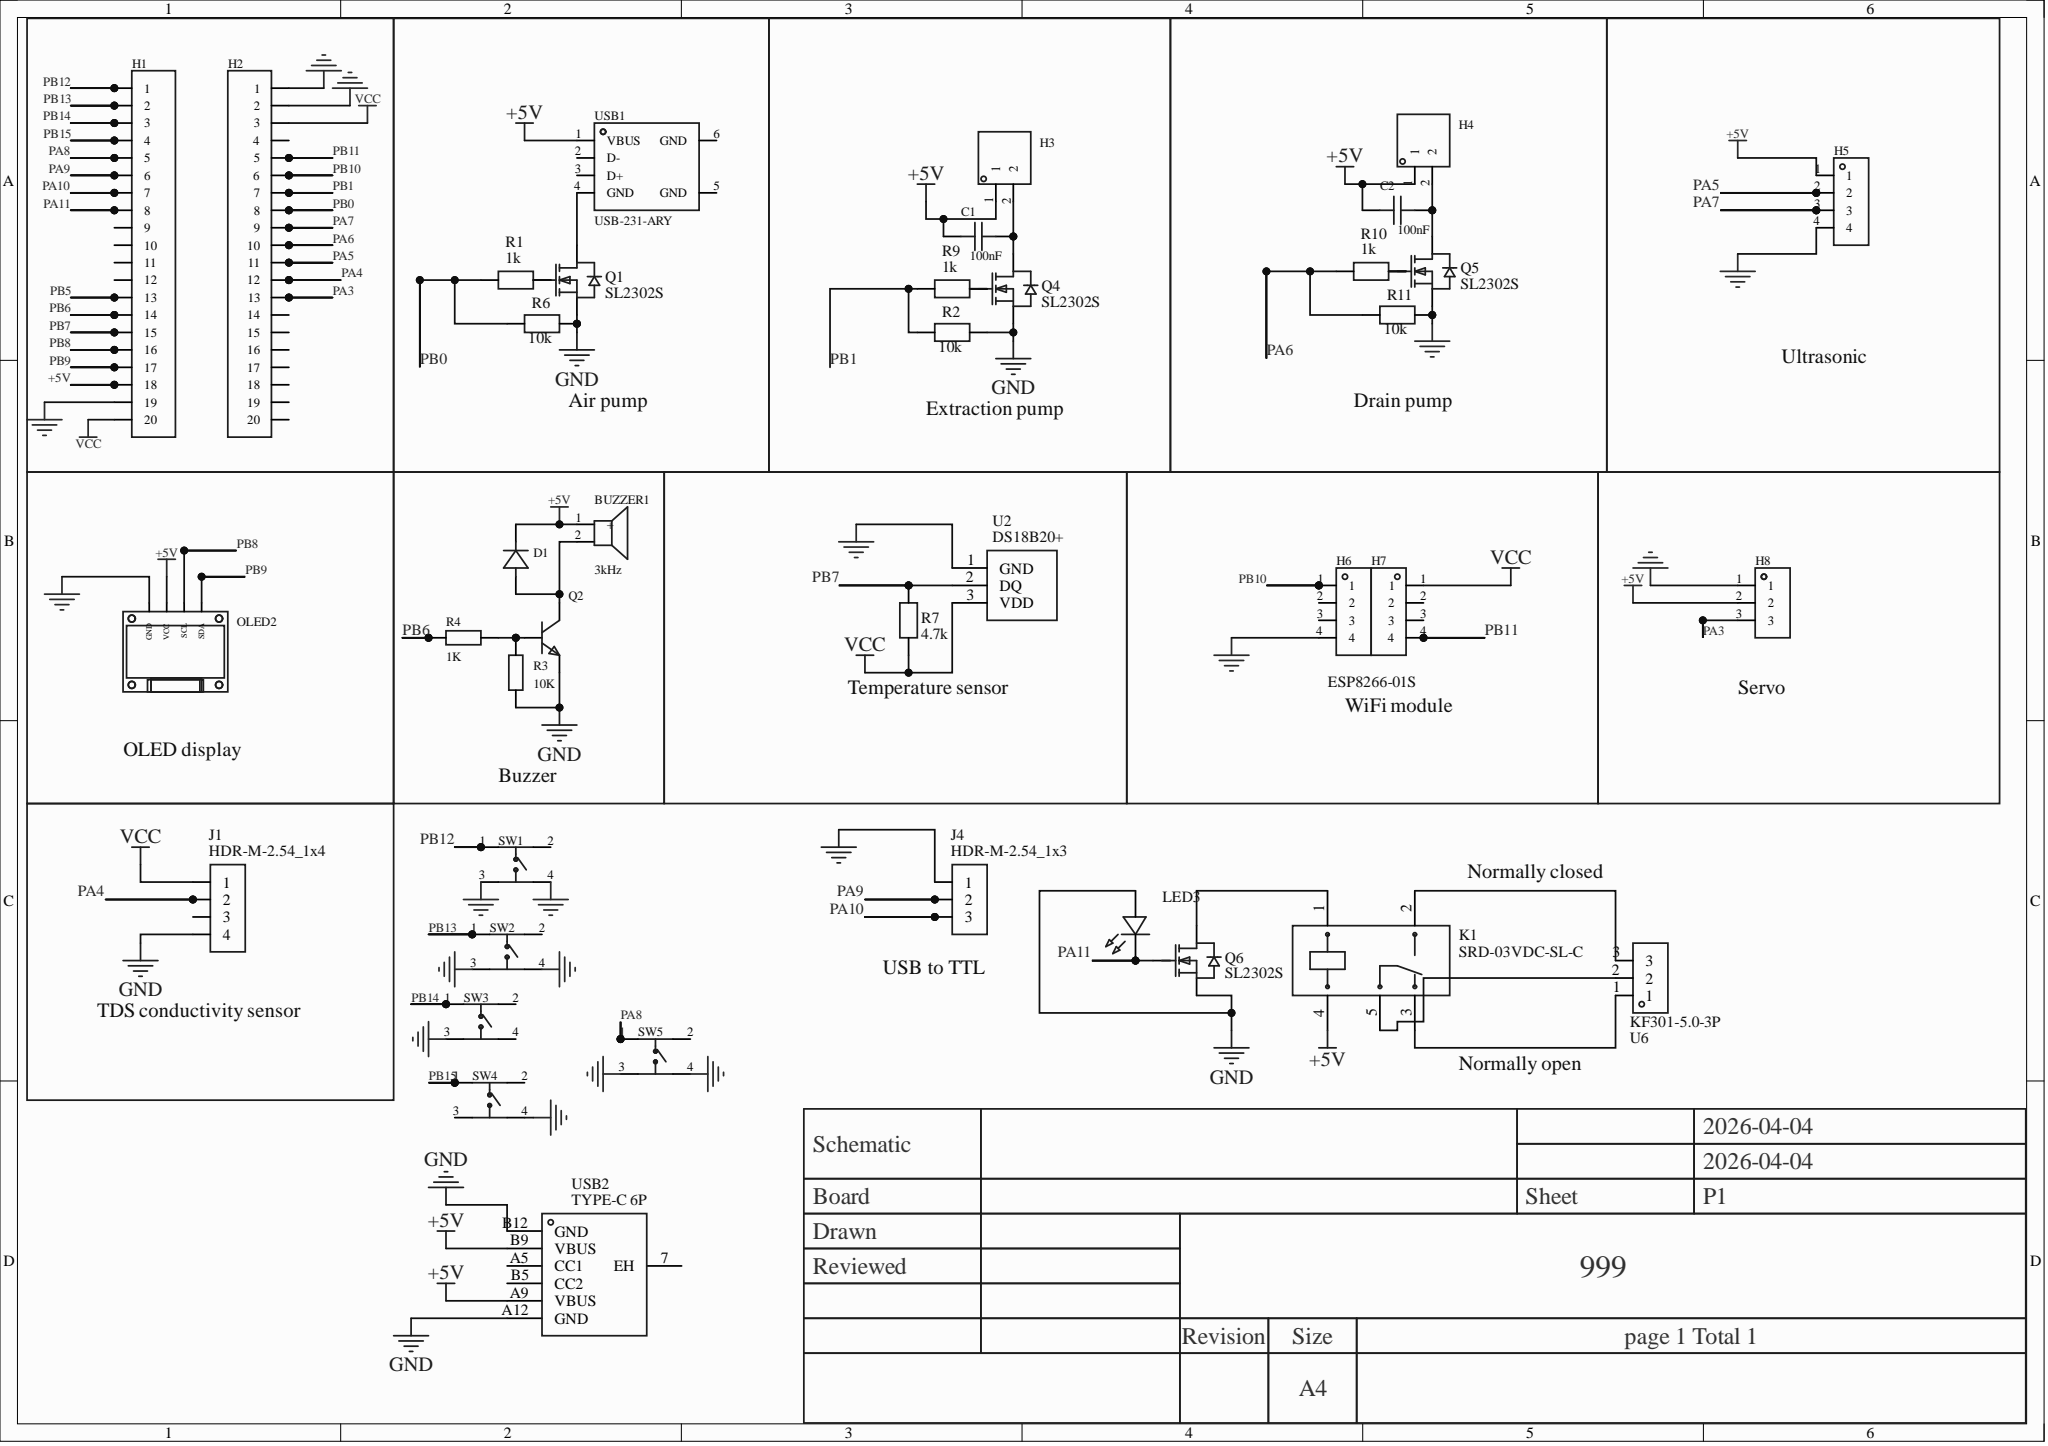Circuit board | Altium Designer | 40 parts | 36 nets
Bill of materials:
Comment,Description,Designator,Footprint,LibRef,Quantity
"3kHz","Drive method: active (built-in driver circuit); Construction type: electromagnetic; Rated voltage: -; Frequency: 3kHz; Sound pressure (SPL): 85dB;","BUZZER1","BUZ-TH_BD9.6-P5.00-D0.7-FD","HNB09A05","1"
"100nF","","C1, C2","C0805","CAP_0805","2"
"","","D1","DO_1N4007","D_1N4007A","1"
"","","H1, H2","HDR-TH_20P-P2.54-V-F","HDR-F_2.54_1x20P","2"
"","","H3, H4","HDR-TH_2P-P2.54-V-M-1","HDR-M_2.54_1x2P","2"
"","","H5, H6, H7","HDR-TH_4P-P2.54-V-M","HDR-M_2.54_1x4P","3"
"","","H8","HDR-TH_3P-P2.54-V-M","HDR-M_2.54_1x3P","1"
"HDR-M-2.54_1x4","","J1","HDR-M-2.54_1X4","HDR-M-2.54_1x4","1"
"HDR-M-2.54_1x3","","J4","HDR-M-2.54_1X3","HDR-M-2.54_1x3","1"
"SRD-03VDC-SL-C","","K1","RELAY-TH_SRD-XXVDC-XL-C","SRD-03VDC-SL-C","1"
"LED-TH-5mm_R","","LED3","LED-TH_BD5.0_RED","LED-TH-5mm_R","1"
"","","OLED2","0.96OLED_4P","0.96OLED模块_4P","1"
"SL2302S","","Q1, Q4, Q5, Q6","SOT-23_L2.9-W1.3-P1.90-LS2.4-BR","SL2302S","4"
"","","Q2","S8050_TO_92","S8050_TO_NPN","1"
"1k","","R1, R4, R9, R10","R0603","1k, Res_0603","4"
"10k","","R2, R3, R6, R11","R0603","10k, Res_0603","4"
"4.7k","","R7","R0603","10k","1"
"J1L0503110","Circuit structure: SPST; Button shape: round button; Actuating force: 2.6N; Mounting: through-hole; Switch length: 6mm; Switch width: 6mm; Switch height: 5mm; With bracket: -; Contact current: 50mA; Rated voltage: 12V; With lamp: none; Operating life: 10万 cycles;","SW1, SW2, SW3, SW4, SW5","SW-TH_4P-L6.0-W6.0-P4.50-LS6.3","J1L0503110","5"
"DS18B20+","","U2","HDR-TH_3P-P2.54-V-F","DS18B20+","1"
"KF301-5.0-3P","","U6","CONN-TH_3P-P5.00_KF301-5.0-3P","KF301-5.0-3P","1"
"USB-231-ARY","Connector type: Type-A; Protocol standard: USB 2.0; Gender: female; Mounting: right angle; Contacts: 4P; Ports: 1; Rated current - power: 1.5A; Operating temperature: -20℃~+70℃;","USB1","USB-A-TH_USB-231-ARY","USB-231-ARY","1"
"TYPE-C 6P","","USB2","TYPE-C-SMD_TYPE-C-6P_1","TYPE-C 6P","1"
Netlist (Protel format):
[
BUZZER1
BUZ-TH_BD9.6-P5.00-D0.7-FD
3kHz



]
[
C1
C0805
100nF



]
[
C2
C0805
100nF



]
[
D1
DO_1N4007




]
[
H1
HDR-TH_20P-P2.54-V-F




]
[
H2
HDR-TH_20P-P2.54-V-F




]
[
H3
HDR-TH_2P-P2.54-V-M-1




]
[
H4
HDR-TH_2P-P2.54-V-M-1




]
[
H5
HDR-TH_4P-P2.54-V-M




]
[
H6
HDR-TH_4P-P2.54-V-M




]
[
H7
HDR-TH_4P-P2.54-V-M




]
[
H8
HDR-TH_3P-P2.54-V-M




]
[
J1
HDR-M-2.54_1X4
HDR-M-2.54_1x4



]
[
J4
HDR-M-2.54_1X3
HDR-M-2.54_1x3



]
[
K1
RELAY-TH_SRD-XXVDC-XL-C
SRD-03VDC-SL-C



]
[
LED3
LED-TH_BD5.0_RED
LED-TH-5mm_R



]
[
OLED2
0.96OLED_4P




]
[
Q1
SOT-23_L2.9-W1.3-P1.90-LS2.4-BR
SL2302S



]
[
Q2
S8050_TO_92




]
[
Q4
SOT-23_L2.9-W1.3-P1.90-LS2.4-BR
SL2302S



]
[
Q5
SOT-23_L2.9-W1.3-P1.90-LS2.4-BR
SL2302S



]
[
Q6
SOT-23_L2.9-W1.3-P1.90-LS2.4-BR
SL2302S



]
[
R1
R0603
1k



]
[
R2
R0603
10k



]
[
R3
R0603
10K



]
[
R4
R0603
1K



]
[
R6
R0603
10k



]
[
R7
R0603
4.7k



]
[
R9
R0603
1k



]
[
R10
R0603
1k



]
[
R11
R0603
10k



]
[
SW1
SW-TH_4P-L6.0-W6.0-P4.50-LS6.3
J1L0503110



]
[
SW2
SW-TH_4P-L6.0-W6.0-P4.50-LS6.3
J1L0503110



]
[
SW3
SW-TH_4P-L6.0-W6.0-P4.50-LS6.3
J1L0503110



]
[
SW4
SW-TH_4P-L6.0-W6.0-P4.50-LS6.3
J1L0503110



]
[
SW5
SW-TH_4P-L6.0-W6.0-P4.50-LS6.3
J1L0503110



]
[
U2
HDR-TH_3P-P2.54-V-F
DS18B20+



]
[
U6
CONN-TH_3P-P5.00_KF301-5.0-3P
KF301-5.0-3P



]
[
USB1
USB-A-TH_USB-231-ARY
USB-231-ARY



]
[
USB2
TYPE-C-SMD_TYPE-C-6P_1
TYPE-C 6P



]
(
VCC
H1-20
H2-3
H7-1
J1-1
R7-2
U2-3
)
(
PB15
H1-4
SW4-1
)
(
PB14
H1-3
SW3-1
)
(
PB13
H1-2
SW2-1
)
(
PB12
H1-1
SW1-1
)
(
PB11
H2-5
H7-4
)
(
PB10
H2-6
H6-1
)
(
PB9
H1-17
OLED2-4
)
(
PB8
H1-16
OLED2-3
)
(
PB7
H1-15
R7-1
U2-2
)
(
PB6
H1-14
R4-2
)
(
PB1
H2-7
R2-1
R9-1
)
(
PB0
H2-8
R1-1
R6-1
)
(
PA11
H1-8
LED3-2
Q6-1
)
(
PA10
H1-7
J4-3
)
(
PA9
H1-6
J4-2
)
(
PA8
H1-5
SW5-1
)
(
PA7
H2-9
H5-3
)
(
PA6
H2-10
R10-1
R11-1
)
(
PA5
H2-11
H5-2
)
(
PA4
H2-12
J1-2
)
(
PA3
H2-13
H8-3
)
(
NetQ5_1
Q5-1
R10-2
)
(
NetQ4_1
Q4-1
R9-2
)
(
NetQ2_2
Q2-2
R3-2
R4-1
)
(
NetQ1_3
Q1-3
USB1-4
)
(
NetQ1_1
Q1-1
R1-2
)
(
NetK1_5
K1-5
U6-2
)
(
NetK1_3
K1-3
U6-1
)
(
NetK1_2
K1-2
U6-3
)
(
NetK1_1
K1-1
Q6-3
)
(
NetC2_2
C2-2
H4-2
Q5-3
)
(
NetC1_2
C1-2
H3-2
Q4-3
)
(
NetBUZZER1_2
BUZZER1-2
D1-2
Q2-3
)
(
GND
H1-19
H2-1
H2-2
H5-4
H6-4
H8-1
J1-4
J4-1
LED3-1
OLED2-1
Q1-2
Q2-1
Q4-2
Q5-2
Q6-2
R2-2
R3-1
R6-2
R11-2
SW1-3
SW1-4
SW2-3
SW2-4
SW3-3
SW4-4
SW5-3
SW5-4
U2-1
USB2-A12
USB2-B12
)
(
+5V
BUZZER1-1
C1-1
C2-1
D1-1
H1-18
H3-1
H4-1
H5-1
H8-2
K1-4
OLED2-2
USB1-1
USB2-A9
USB2-B9
)